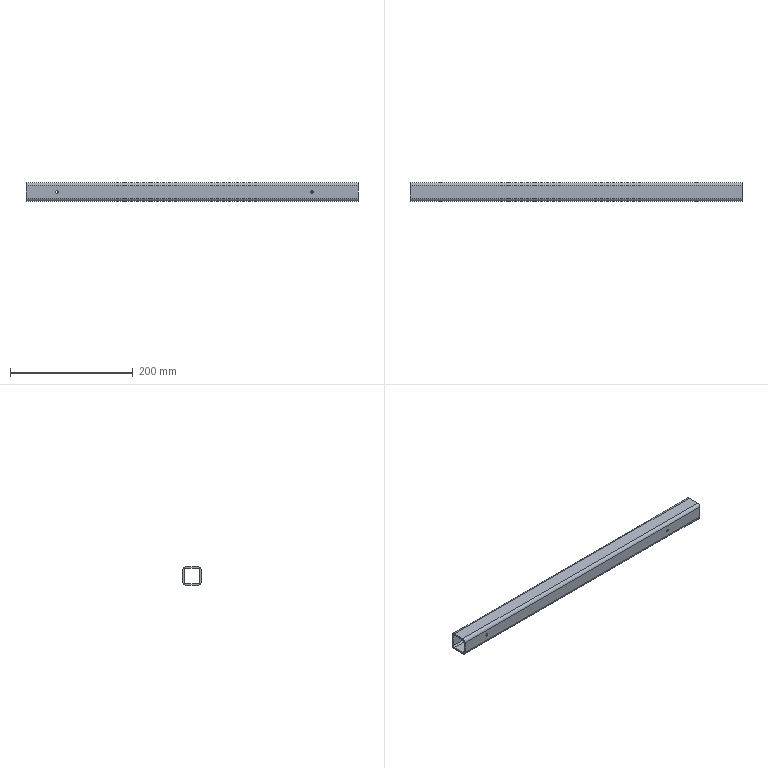Part | SolidWorks | features HoleWzd 2, 3DProfileFeature 1, WeldMemberFeat 1, WeldmentFeature 1 | 1 solid | 26 faces | box 540 x 30 x 30 mm | volume 144334 mm3 | cylinder 16 | plane 10 | commonest cylinder face diameters 4.2 x8 5.2 x4 10.4 x4
STEP:
#1=CARTESIAN_POINT('',(50.,15.,2.1));
#2=VERTEX_POINT('',#1);
#3=CARTESIAN_POINT('',(50.,15.,-2.1));
#4=VERTEX_POINT('',#3);
#5=CARTESIAN_POINT('',(50.,15.,0.));
#6=DIRECTION('',(0.,-1.,0.));
#7=DIRECTION('',(0.,0.,-1.));
#8=AXIS2_PLACEMENT_3D('',#5,#6,#7);
#9=CIRCLE('',#8,2.1);
#10=EDGE_CURVE('',#2,#4,#9,.T.);
#11=ORIENTED_EDGE('',*,*,#10,.F.);
#12=CARTESIAN_POINT('',(50.,12.4,2.1));
#13=VERTEX_POINT('',#12);
#14=CARTESIAN_POINT('',(50.,-15.,2.1));
#15=DIRECTION('',(0.,-1.,0.));
#16=VECTOR('',#15,1000.);
#17=LINE('',#14,#16);
#18=EDGE_CURVE('',#2,#13,#17,.T.);
#19=ORIENTED_EDGE('',*,*,#18,.T.);
#20=CARTESIAN_POINT('',(50.,12.4,-2.1));
#21=VERTEX_POINT('',#20);
#22=CARTESIAN_POINT('',(50.,12.4,0.));
#23=DIRECTION('',(0.,-1.,0.));
#24=DIRECTION('',(0.,0.,-1.));
#25=AXIS2_PLACEMENT_3D('',#22,#23,#24);
#26=CIRCLE('',#25,2.1);
#27=EDGE_CURVE('',#13,#21,#26,.T.);
#28=ORIENTED_EDGE('',*,*,#27,.T.);
#29=CARTESIAN_POINT('',(50.,-15.,-2.1));
#30=DIRECTION('',(0.,-1.,0.));
#31=VECTOR('',#30,1000.);
#32=LINE('',#29,#31);
#33=EDGE_CURVE('',#4,#21,#32,.T.);
#34=ORIENTED_EDGE('',*,*,#33,.F.);
#35=EDGE_LOOP('',(#11,#19,#28,#34));
#36=FACE_OUTER_BOUND('',#35,.T.);
#37=CARTESIAN_POINT('',(50.,-15.,0.));
#38=DIRECTION('',(0.,-1.,0.));
#39=DIRECTION('',(0.,0.,-1.));
#40=AXIS2_PLACEMENT_3D('',#37,#38,#39);
#41=CYLINDRICAL_SURFACE('',#40,2.1);
#42=ADVANCED_FACE('',(#36),#41,.F.);
#43=CARTESIAN_POINT('',(50.,-12.4,-2.1));
#44=VERTEX_POINT('',#43);
#45=CARTESIAN_POINT('',(50.,-12.4,2.1));
#46=VERTEX_POINT('',#45);
#47=CARTESIAN_POINT('',(50.,-12.4,0.));
#48=DIRECTION('',(0.,1.,0.));
#49=DIRECTION('',(0.,0.,1.));
#50=AXIS2_PLACEMENT_3D('',#47,#48,#49);
#51=CIRCLE('',#50,2.1);
#52=EDGE_CURVE('',#44,#46,#51,.T.);
#53=ORIENTED_EDGE('',*,*,#52,.T.);
#54=CARTESIAN_POINT('',(50.,-15.,2.1));
#55=VERTEX_POINT('',#54);
#56=CARTESIAN_POINT('',(50.,-15.,2.1));
#57=DIRECTION('',(0.,-1.,0.));
#58=VECTOR('',#57,1000.);
#59=LINE('',#56,#58);
#60=EDGE_CURVE('',#46,#55,#59,.T.);
#61=ORIENTED_EDGE('',*,*,#60,.T.);
#62=CARTESIAN_POINT('',(50.,-15.,-2.1));
#63=VERTEX_POINT('',#62);
#64=CARTESIAN_POINT('',(50.,-15.,0.));
#65=DIRECTION('',(0.,-1.,0.));
#66=DIRECTION('',(0.,0.,-1.));
#67=AXIS2_PLACEMENT_3D('',#64,#65,#66);
#68=CIRCLE('',#67,2.1);
#69=EDGE_CURVE('',#55,#63,#68,.T.);
#70=ORIENTED_EDGE('',*,*,#69,.T.);
#71=CARTESIAN_POINT('',(50.,-15.,-2.1));
#72=DIRECTION('',(0.,-1.,0.));
#73=VECTOR('',#72,1000.);
#74=LINE('',#71,#73);
#75=EDGE_CURVE('',#44,#63,#74,.T.);
#76=ORIENTED_EDGE('',*,*,#75,.F.);
#77=EDGE_LOOP('',(#53,#61,#70,#76));
#78=FACE_OUTER_BOUND('',#77,.T.);
#79=CARTESIAN_POINT('',(50.,-15.,0.));
#80=DIRECTION('',(0.,-1.,0.));
#81=DIRECTION('',(0.,0.,-1.));
#82=AXIS2_PLACEMENT_3D('',#79,#80,#81);
#83=CYLINDRICAL_SURFACE('',#82,2.1);
#84=ADVANCED_FACE('',(#78),#83,.F.);
#85=CARTESIAN_POINT('',(465.,15.,2.1));
#86=VERTEX_POINT('',#85);
#87=CARTESIAN_POINT('',(465.,15.,-2.1));
#88=VERTEX_POINT('',#87);
#89=CARTESIAN_POINT('',(465.,15.,0.));
#90=DIRECTION('',(0.,-1.,0.));
#91=DIRECTION('',(0.,0.,-1.));
#92=AXIS2_PLACEMENT_3D('',#89,#90,#91);
#93=CIRCLE('',#92,2.1);
#94=EDGE_CURVE('',#86,#88,#93,.T.);
#95=ORIENTED_EDGE('',*,*,#94,.F.);
#96=CARTESIAN_POINT('',(465.,12.4,2.1));
#97=VERTEX_POINT('',#96);
#98=CARTESIAN_POINT('',(465.,-15.,2.1));
#99=DIRECTION('',(0.,-1.,0.));
#100=VECTOR('',#99,1000.);
#101=LINE('',#98,#100);
#102=EDGE_CURVE('',#86,#97,#101,.T.);
#103=ORIENTED_EDGE('',*,*,#102,.T.);
#104=CARTESIAN_POINT('',(465.,12.4,-2.1));
#105=VERTEX_POINT('',#104);
#106=CARTESIAN_POINT('',(465.,12.4,0.));
#107=DIRECTION('',(0.,-1.,0.));
#108=DIRECTION('',(0.,0.,-1.));
#109=AXIS2_PLACEMENT_3D('',#106,#107,#108);
#110=CIRCLE('',#109,2.1);
#111=EDGE_CURVE('',#97,#105,#110,.T.);
#112=ORIENTED_EDGE('',*,*,#111,.T.);
#113=CARTESIAN_POINT('',(465.,-15.,-2.1));
#114=DIRECTION('',(0.,-1.,0.));
#115=VECTOR('',#114,1000.);
#116=LINE('',#113,#115);
#117=EDGE_CURVE('',#88,#105,#116,.T.);
#118=ORIENTED_EDGE('',*,*,#117,.F.);
#119=EDGE_LOOP('',(#95,#103,#112,#118));
#120=FACE_OUTER_BOUND('',#119,.T.);
#121=CARTESIAN_POINT('',(465.,-15.,0.));
#122=DIRECTION('',(0.,-1.,0.));
#123=DIRECTION('',(0.,0.,-1.));
#124=AXIS2_PLACEMENT_3D('',#121,#122,#123);
#125=CYLINDRICAL_SURFACE('',#124,2.1);
#126=ADVANCED_FACE('',(#120),#125,.F.);
#127=CARTESIAN_POINT('',(465.,-12.4,-2.1));
#128=VERTEX_POINT('',#127);
#129=CARTESIAN_POINT('',(465.,-12.4,2.1));
#130=VERTEX_POINT('',#129);
#131=CARTESIAN_POINT('',(465.,-12.4,0.));
#132=DIRECTION('',(0.,1.,0.));
#133=DIRECTION('',(0.,0.,1.));
#134=AXIS2_PLACEMENT_3D('',#131,#132,#133);
#135=CIRCLE('',#134,2.1);
#136=EDGE_CURVE('',#128,#130,#135,.T.);
#137=ORIENTED_EDGE('',*,*,#136,.T.);
#138=CARTESIAN_POINT('',(465.,-15.,2.1));
#139=VERTEX_POINT('',#138);
#140=CARTESIAN_POINT('',(465.,-15.,2.1));
#141=DIRECTION('',(0.,-1.,0.));
#142=VECTOR('',#141,1000.);
#143=LINE('',#140,#142);
#144=EDGE_CURVE('',#130,#139,#143,.T.);
#145=ORIENTED_EDGE('',*,*,#144,.T.);
#146=CARTESIAN_POINT('',(465.,-15.,-2.1));
#147=VERTEX_POINT('',#146);
#148=CARTESIAN_POINT('',(465.,-15.,0.));
#149=DIRECTION('',(0.,-1.,0.));
#150=DIRECTION('',(0.,0.,-1.));
#151=AXIS2_PLACEMENT_3D('',#148,#149,#150);
#152=CIRCLE('',#151,2.1);
#153=EDGE_CURVE('',#139,#147,#152,.T.);
#154=ORIENTED_EDGE('',*,*,#153,.T.);
#155=CARTESIAN_POINT('',(465.,-15.,-2.1));
#156=DIRECTION('',(0.,-1.,0.));
#157=VECTOR('',#156,1000.);
#158=LINE('',#155,#157);
#159=EDGE_CURVE('',#128,#147,#158,.T.);
#160=ORIENTED_EDGE('',*,*,#159,.F.);
#161=EDGE_LOOP('',(#137,#145,#154,#160));
#162=FACE_OUTER_BOUND('',#161,.T.);
#163=CARTESIAN_POINT('',(465.,-15.,0.));
#164=DIRECTION('',(0.,-1.,0.));
#165=DIRECTION('',(0.,0.,-1.));
#166=AXIS2_PLACEMENT_3D('',#163,#164,#165);
#167=CYLINDRICAL_SURFACE('',#166,2.1);
#168=ADVANCED_FACE('',(#162),#167,.F.);
#169=CARTESIAN_POINT('',(0.,9.8,-15.));
#170=VERTEX_POINT('',#169);
#171=CARTESIAN_POINT('',(0.,15.,-9.8));
#172=VERTEX_POINT('',#171);
#173=CARTESIAN_POINT('',(0.,9.8,-9.8));
#174=DIRECTION('',(1.,0.,0.));
#175=DIRECTION('',(0.,0.,-1.));
#176=AXIS2_PLACEMENT_3D('',#173,#174,#175);
#177=CIRCLE('',#176,5.2);
#178=EDGE_CURVE('',#170,#172,#177,.T.);
#179=ORIENTED_EDGE('',*,*,#178,.T.);
#180=CARTESIAN_POINT('',(540.,15.,-9.8));
#181=VERTEX_POINT('',#180);
#182=CARTESIAN_POINT('',(540.,15.,-9.8));
#183=DIRECTION('',(-1.,0.,0.));
#184=VECTOR('',#183,1000.);
#185=LINE('',#182,#184);
#186=EDGE_CURVE('',#181,#172,#185,.T.);
#187=ORIENTED_EDGE('',*,*,#186,.F.);
#188=CARTESIAN_POINT('',(540.,9.8,-15.));
#189=VERTEX_POINT('',#188);
#190=CARTESIAN_POINT('',(540.,9.8,-9.8));
#191=DIRECTION('',(1.,0.,0.));
#192=DIRECTION('',(0.,0.,-1.));
#193=AXIS2_PLACEMENT_3D('',#190,#191,#192);
#194=CIRCLE('',#193,5.2);
#195=EDGE_CURVE('',#189,#181,#194,.T.);
#196=ORIENTED_EDGE('',*,*,#195,.F.);
#197=CARTESIAN_POINT('',(540.,9.8,-15.));
#198=DIRECTION('',(-1.,0.,0.));
#199=VECTOR('',#198,1000.);
#200=LINE('',#197,#199);
#201=EDGE_CURVE('',#189,#170,#200,.T.);
#202=ORIENTED_EDGE('',*,*,#201,.T.);
#203=EDGE_LOOP('',(#179,#187,#196,#202));
#204=FACE_OUTER_BOUND('',#203,.T.);
#205=CARTESIAN_POINT('',(540.,9.8,-9.8));
#206=DIRECTION('',(-1.,0.,0.));
#207=DIRECTION('',(0.,0.,1.));
#208=AXIS2_PLACEMENT_3D('',#205,#206,#207);
#209=CYLINDRICAL_SURFACE('',#208,5.2);
#210=ADVANCED_FACE('',(#204),#209,.T.);
#211=CARTESIAN_POINT('',(50.,15.,0.));
#212=DIRECTION('',(0.,-1.,0.));
#213=DIRECTION('',(0.,0.,-1.));
#214=AXIS2_PLACEMENT_3D('',#211,#212,#213);
#215=CIRCLE('',#214,2.1);
#216=EDGE_CURVE('',#4,#2,#215,.T.);
#217=ORIENTED_EDGE('',*,*,#216,.T.);
#218=ORIENTED_EDGE('',*,*,#10,.T.);
#219=EDGE_LOOP('',(#217,#218));
#220=FACE_BOUND('',#219,.T.);
#221=CARTESIAN_POINT('',(465.,15.,0.));
#222=DIRECTION('',(0.,-1.,0.));
#223=DIRECTION('',(0.,0.,-1.));
#224=AXIS2_PLACEMENT_3D('',#221,#222,#223);
#225=CIRCLE('',#224,2.1);
#226=EDGE_CURVE('',#88,#86,#225,.T.);
#227=ORIENTED_EDGE('',*,*,#226,.T.);
#228=ORIENTED_EDGE('',*,*,#94,.T.);
#229=EDGE_LOOP('',(#227,#228));
#230=FACE_BOUND('',#229,.T.);
#231=CARTESIAN_POINT('',(0.,15.,9.8));
#232=VERTEX_POINT('',#231);
#233=CARTESIAN_POINT('',(0.,15.,-9.8));
#234=DIRECTION('',(0.,0.,1.));
#235=VECTOR('',#234,1000.);
#236=LINE('',#233,#235);
#237=EDGE_CURVE('',#172,#232,#236,.T.);
#238=ORIENTED_EDGE('',*,*,#237,.T.);
#239=CARTESIAN_POINT('',(540.,15.,9.8));
#240=VERTEX_POINT('',#239);
#241=CARTESIAN_POINT('',(540.,15.,9.8));
#242=DIRECTION('',(-1.,0.,0.));
#243=VECTOR('',#242,1000.);
#244=LINE('',#241,#243);
#245=EDGE_CURVE('',#240,#232,#244,.T.);
#246=ORIENTED_EDGE('',*,*,#245,.F.);
#247=CARTESIAN_POINT('',(540.,15.,-9.8));
#248=DIRECTION('',(0.,0.,1.));
#249=VECTOR('',#248,1000.);
#250=LINE('',#247,#249);
#251=EDGE_CURVE('',#181,#240,#250,.T.);
#252=ORIENTED_EDGE('',*,*,#251,.F.);
#253=ORIENTED_EDGE('',*,*,#186,.T.);
#254=EDGE_LOOP('',(#238,#246,#252,#253));
#255=FACE_OUTER_BOUND('',#254,.T.);
#256=CARTESIAN_POINT('',(540.,15.,-9.8));
#257=DIRECTION('',(0.,-1.,0.));
#258=DIRECTION('',(0.,0.,-1.));
#259=AXIS2_PLACEMENT_3D('',#256,#257,#258);
#260=PLANE('',#259);
#261=ADVANCED_FACE('',(#220,#230,#255),#260,.F.);
#262=CARTESIAN_POINT('',(0.,9.8,15.));
#263=VERTEX_POINT('',#262);
#264=CARTESIAN_POINT('',(0.,9.8,9.8));
#265=DIRECTION('',(1.,0.,0.));
#266=DIRECTION('',(0.,0.,-1.));
#267=AXIS2_PLACEMENT_3D('',#264,#265,#266);
#268=CIRCLE('',#267,5.2);
#269=EDGE_CURVE('',#232,#263,#268,.T.);
#270=ORIENTED_EDGE('',*,*,#269,.T.);
#271=CARTESIAN_POINT('',(540.,9.8,15.));
#272=VERTEX_POINT('',#271);
#273=CARTESIAN_POINT('',(540.,9.8,15.));
#274=DIRECTION('',(-1.,0.,0.));
#275=VECTOR('',#274,1000.);
#276=LINE('',#273,#275);
#277=EDGE_CURVE('',#272,#263,#276,.T.);
#278=ORIENTED_EDGE('',*,*,#277,.F.);
#279=CARTESIAN_POINT('',(540.,9.8,9.8));
#280=DIRECTION('',(1.,0.,0.));
#281=DIRECTION('',(0.,0.,-1.));
#282=AXIS2_PLACEMENT_3D('',#279,#280,#281);
#283=CIRCLE('',#282,5.2);
#284=EDGE_CURVE('',#240,#272,#283,.T.);
#285=ORIENTED_EDGE('',*,*,#284,.F.);
#286=ORIENTED_EDGE('',*,*,#245,.T.);
#287=EDGE_LOOP('',(#270,#278,#285,#286));
#288=FACE_OUTER_BOUND('',#287,.T.);
#289=CARTESIAN_POINT('',(540.,9.8,9.8));
#290=DIRECTION('',(-1.,0.,0.));
#291=DIRECTION('',(0.,0.,1.));
#292=AXIS2_PLACEMENT_3D('',#289,#290,#291);
#293=CYLINDRICAL_SURFACE('',#292,5.2);
#294=ADVANCED_FACE('',(#288),#293,.T.);
#295=CARTESIAN_POINT('',(0.,-9.8,15.));
#296=VERTEX_POINT('',#295);
#297=CARTESIAN_POINT('',(0.,-9.8,15.));
#298=DIRECTION('',(0.,-1.,0.));
#299=VECTOR('',#298,1000.);
#300=LINE('',#297,#299);
#301=EDGE_CURVE('',#263,#296,#300,.T.);
#302=ORIENTED_EDGE('',*,*,#301,.T.);
#303=CARTESIAN_POINT('',(540.,-9.8,15.));
#304=VERTEX_POINT('',#303);
#305=CARTESIAN_POINT('',(540.,-9.8,15.));
#306=DIRECTION('',(-1.,0.,0.));
#307=VECTOR('',#306,1000.);
#308=LINE('',#305,#307);
#309=EDGE_CURVE('',#304,#296,#308,.T.);
#310=ORIENTED_EDGE('',*,*,#309,.F.);
#311=CARTESIAN_POINT('',(540.,-9.8,15.));
#312=DIRECTION('',(0.,-1.,0.));
#313=VECTOR('',#312,1000.);
#314=LINE('',#311,#313);
#315=EDGE_CURVE('',#272,#304,#314,.T.);
#316=ORIENTED_EDGE('',*,*,#315,.F.);
#317=ORIENTED_EDGE('',*,*,#277,.T.);
#318=EDGE_LOOP('',(#302,#310,#316,#317));
#319=FACE_OUTER_BOUND('',#318,.T.);
#320=CARTESIAN_POINT('',(540.,-9.8,15.));
#321=DIRECTION('',(0.,0.,-1.));
#322=DIRECTION('',(-1.,0.,0.));
#323=AXIS2_PLACEMENT_3D('',#320,#321,#322);
#324=PLANE('',#323);
#325=ADVANCED_FACE('',(#319),#324,.F.);
#326=CARTESIAN_POINT('',(0.,-15.,9.8));
#327=VERTEX_POINT('',#326);
#328=CARTESIAN_POINT('',(0.,-9.8,9.8));
#329=DIRECTION('',(1.,0.,0.));
#330=DIRECTION('',(0.,0.,-1.));
#331=AXIS2_PLACEMENT_3D('',#328,#329,#330);
#332=CIRCLE('',#331,5.2);
#333=EDGE_CURVE('',#296,#327,#332,.T.);
#334=ORIENTED_EDGE('',*,*,#333,.T.);
#335=CARTESIAN_POINT('',(540.,-15.,9.8));
#336=VERTEX_POINT('',#335);
#337=CARTESIAN_POINT('',(540.,-15.,9.8));
#338=DIRECTION('',(-1.,0.,0.));
#339=VECTOR('',#338,1000.);
#340=LINE('',#337,#339);
#341=EDGE_CURVE('',#336,#327,#340,.T.);
#342=ORIENTED_EDGE('',*,*,#341,.F.);
#343=CARTESIAN_POINT('',(540.,-9.8,9.8));
#344=DIRECTION('',(1.,0.,0.));
#345=DIRECTION('',(0.,0.,-1.));
#346=AXIS2_PLACEMENT_3D('',#343,#344,#345);
#347=CIRCLE('',#346,5.2);
#348=EDGE_CURVE('',#304,#336,#347,.T.);
#349=ORIENTED_EDGE('',*,*,#348,.F.);
#350=ORIENTED_EDGE('',*,*,#309,.T.);
#351=EDGE_LOOP('',(#334,#342,#349,#350));
#352=FACE_OUTER_BOUND('',#351,.T.);
#353=CARTESIAN_POINT('',(540.,-9.8,9.8));
#354=DIRECTION('',(-1.,0.,0.));
#355=DIRECTION('',(0.,0.,1.));
#356=AXIS2_PLACEMENT_3D('',#353,#354,#355);
#357=CYLINDRICAL_SURFACE('',#356,5.2);
#358=ADVANCED_FACE('',(#352),#357,.T.);
#359=CARTESIAN_POINT('',(50.,-15.,0.));
#360=DIRECTION('',(0.,-1.,0.));
#361=DIRECTION('',(0.,0.,-1.));
#362=AXIS2_PLACEMENT_3D('',#359,#360,#361);
#363=CIRCLE('',#362,2.1);
#364=EDGE_CURVE('',#63,#55,#363,.T.);
#365=ORIENTED_EDGE('',*,*,#364,.F.);
#366=ORIENTED_EDGE('',*,*,#69,.F.);
#367=EDGE_LOOP('',(#365,#366));
#368=FACE_BOUND('',#367,.T.);
#369=CARTESIAN_POINT('',(465.,-15.,0.));
#370=DIRECTION('',(0.,-1.,0.));
#371=DIRECTION('',(0.,0.,-1.));
#372=AXIS2_PLACEMENT_3D('',#369,#370,#371);
#373=CIRCLE('',#372,2.1);
#374=EDGE_CURVE('',#147,#139,#373,.T.);
#375=ORIENTED_EDGE('',*,*,#374,.F.);
#376=ORIENTED_EDGE('',*,*,#153,.F.);
#377=EDGE_LOOP('',(#375,#376));
#378=FACE_BOUND('',#377,.T.);
#379=CARTESIAN_POINT('',(0.,-15.,-9.8));
#380=VERTEX_POINT('',#379);
#381=CARTESIAN_POINT('',(0.,-15.,9.8));
#382=DIRECTION('',(0.,0.,-1.));
#383=VECTOR('',#382,1000.);
#384=LINE('',#381,#383);
#385=EDGE_CURVE('',#327,#380,#384,.T.);
#386=ORIENTED_EDGE('',*,*,#385,.T.);
#387=CARTESIAN_POINT('',(540.,-15.,-9.8));
#388=VERTEX_POINT('',#387);
#389=CARTESIAN_POINT('',(540.,-15.,-9.8));
#390=DIRECTION('',(-1.,0.,0.));
#391=VECTOR('',#390,1000.);
#392=LINE('',#389,#391);
#393=EDGE_CURVE('',#388,#380,#392,.T.);
#394=ORIENTED_EDGE('',*,*,#393,.F.);
#395=CARTESIAN_POINT('',(540.,-15.,9.8));
#396=DIRECTION('',(0.,0.,-1.));
#397=VECTOR('',#396,1000.);
#398=LINE('',#395,#397);
#399=EDGE_CURVE('',#336,#388,#398,.T.);
#400=ORIENTED_EDGE('',*,*,#399,.F.);
#401=ORIENTED_EDGE('',*,*,#341,.T.);
#402=EDGE_LOOP('',(#386,#394,#400,#401));
#403=FACE_OUTER_BOUND('',#402,.T.);
#404=CARTESIAN_POINT('',(540.,-15.,9.8));
#405=DIRECTION('',(0.,1.,0.));
#406=DIRECTION('',(0.,0.,1.));
#407=AXIS2_PLACEMENT_3D('',#404,#405,#406);
#408=PLANE('',#407);
#409=ADVANCED_FACE('',(#368,#378,#403),#408,.F.);
#410=CARTESIAN_POINT('',(0.,-9.8,-15.));
#411=VERTEX_POINT('',#410);
#412=CARTESIAN_POINT('',(0.,-9.8,-9.8));
#413=DIRECTION('',(1.,0.,0.));
#414=DIRECTION('',(0.,0.,-1.));
#415=AXIS2_PLACEMENT_3D('',#412,#413,#414);
#416=CIRCLE('',#415,5.2);
#417=EDGE_CURVE('',#380,#411,#416,.T.);
#418=ORIENTED_EDGE('',*,*,#417,.T.);
#419=CARTESIAN_POINT('',(540.,-9.8,-15.));
#420=VERTEX_POINT('',#419);
#421=CARTESIAN_POINT('',(540.,-9.8,-15.));
#422=DIRECTION('',(-1.,0.,0.));
#423=VECTOR('',#422,1000.);
#424=LINE('',#421,#423);
#425=EDGE_CURVE('',#420,#411,#424,.T.);
#426=ORIENTED_EDGE('',*,*,#425,.F.);
#427=CARTESIAN_POINT('',(540.,-9.8,-9.8));
#428=DIRECTION('',(1.,0.,0.));
#429=DIRECTION('',(0.,0.,-1.));
#430=AXIS2_PLACEMENT_3D('',#427,#428,#429);
#431=CIRCLE('',#430,5.2);
#432=EDGE_CURVE('',#388,#420,#431,.T.);
#433=ORIENTED_EDGE('',*,*,#432,.F.);
#434=ORIENTED_EDGE('',*,*,#393,.T.);
#435=EDGE_LOOP('',(#418,#426,#433,#434));
#436=FACE_OUTER_BOUND('',#435,.T.);
#437=CARTESIAN_POINT('',(540.,-9.8,-9.8));
#438=DIRECTION('',(-1.,0.,0.));
#439=DIRECTION('',(0.,0.,1.));
#440=AXIS2_PLACEMENT_3D('',#437,#438,#439);
#441=CYLINDRICAL_SURFACE('',#440,5.2);
#442=ADVANCED_FACE('',(#436),#441,.T.);
#443=CARTESIAN_POINT('',(0.,12.4,9.8));
#444=VERTEX_POINT('',#443);
#445=CARTESIAN_POINT('',(0.,9.8,12.4));
#446=VERTEX_POINT('',#445);
#447=CARTESIAN_POINT('',(0.,9.8,9.8));
#448=DIRECTION('',(1.,0.,0.));
#449=DIRECTION('',(0.,0.,-1.));
#450=AXIS2_PLACEMENT_3D('',#447,#448,#449);
#451=CIRCLE('',#450,2.6);
#452=EDGE_CURVE('',#444,#446,#451,.T.);
#453=ORIENTED_EDGE('',*,*,#452,.F.);
#454=CARTESIAN_POINT('',(540.,12.4,9.8));
#455=VERTEX_POINT('',#454);
#456=CARTESIAN_POINT('',(540.,12.4,9.8));
#457=DIRECTION('',(-1.,0.,0.));
#458=VECTOR('',#457,1000.);
#459=LINE('',#456,#458);
#460=EDGE_CURVE('',#455,#444,#459,.T.);
#461=ORIENTED_EDGE('',*,*,#460,.F.);
#462=CARTESIAN_POINT('',(540.,9.8,12.4));
#463=VERTEX_POINT('',#462);
#464=CARTESIAN_POINT('',(540.,9.8,9.8));
#465=DIRECTION('',(1.,0.,0.));
#466=DIRECTION('',(0.,0.,-1.));
#467=AXIS2_PLACEMENT_3D('',#464,#465,#466);
#468=CIRCLE('',#467,2.6);
#469=EDGE_CURVE('',#455,#463,#468,.T.);
#470=ORIENTED_EDGE('',*,*,#469,.T.);
#471=CARTESIAN_POINT('',(540.,9.8,12.4));
#472=DIRECTION('',(-1.,0.,0.));
#473=VECTOR('',#472,1000.);
#474=LINE('',#471,#473);
#475=EDGE_CURVE('',#463,#446,#474,.T.);
#476=ORIENTED_EDGE('',*,*,#475,.T.);
#477=EDGE_LOOP('',(#453,#461,#470,#476));
#478=FACE_OUTER_BOUND('',#477,.T.);
#479=CARTESIAN_POINT('',(540.,9.8,9.8));
#480=DIRECTION('',(-1.,0.,0.));
#481=DIRECTION('',(0.,0.,1.));
#482=AXIS2_PLACEMENT_3D('',#479,#480,#481);
#483=CYLINDRICAL_SURFACE('',#482,2.6);
#484=ADVANCED_FACE('',(#478),#483,.F.);
#485=CARTESIAN_POINT('',(50.,12.4,0.));
#486=DIRECTION('',(0.,-1.,0.));
#487=DIRECTION('',(0.,0.,-1.));
#488=AXIS2_PLACEMENT_3D('',#485,#486,#487);
#489=CIRCLE('',#488,2.1);
#490=EDGE_CURVE('',#21,#13,#489,.T.);
#491=ORIENTED_EDGE('',*,*,#490,.F.);
#492=ORIENTED_EDGE('',*,*,#27,.F.);
#493=EDGE_LOOP('',(#491,#492));
#494=FACE_BOUND('',#493,.T.);
#495=CARTESIAN_POINT('',(465.,12.4,0.));
#496=DIRECTION('',(0.,-1.,0.));
#497=DIRECTION('',(0.,0.,-1.));
#498=AXIS2_PLACEMENT_3D('',#495,#496,#497);
#499=CIRCLE('',#498,2.1);
#500=EDGE_CURVE('',#105,#97,#499,.T.);
#501=ORIENTED_EDGE('',*,*,#500,.F.);
#502=ORIENTED_EDGE('',*,*,#111,.F.);
#503=EDGE_LOOP('',(#501,#502));
#504=FACE_BOUND('',#503,.T.);
#505=CARTESIAN_POINT('',(0.,12.4,-9.8));
#506=VERTEX_POINT('',#505);
#507=CARTESIAN_POINT('',(0.,12.4,-9.8));
#508=DIRECTION('',(0.,0.,1.));
#509=VECTOR('',#508,1000.);
#510=LINE('',#507,#509);
#511=EDGE_CURVE('',#506,#444,#510,.T.);
#512=ORIENTED_EDGE('',*,*,#511,.F.);
#513=CARTESIAN_POINT('',(540.,12.4,-9.8));
#514=VERTEX_POINT('',#513);
#515=CARTESIAN_POINT('',(540.,12.4,-9.8));
#516=DIRECTION('',(-1.,0.,0.));
#517=VECTOR('',#516,1000.);
#518=LINE('',#515,#517);
#519=EDGE_CURVE('',#514,#506,#518,.T.);
#520=ORIENTED_EDGE('',*,*,#519,.F.);
#521=CARTESIAN_POINT('',(540.,12.4,-9.8));
#522=DIRECTION('',(0.,0.,1.));
#523=VECTOR('',#522,1000.);
#524=LINE('',#521,#523);
#525=EDGE_CURVE('',#514,#455,#524,.T.);
#526=ORIENTED_EDGE('',*,*,#525,.T.);
#527=ORIENTED_EDGE('',*,*,#460,.T.);
#528=EDGE_LOOP('',(#512,#520,#526,#527));
#529=FACE_OUTER_BOUND('',#528,.T.);
#530=CARTESIAN_POINT('',(540.,12.4,-9.8));
#531=DIRECTION('',(0.,-1.,0.));
#532=DIRECTION('',(0.,0.,-1.));
#533=AXIS2_PLACEMENT_3D('',#530,#531,#532);
#534=PLANE('',#533);
#535=ADVANCED_FACE('',(#494,#504,#529),#534,.T.);
#536=CARTESIAN_POINT('',(0.,9.8,-12.4));
#537=VERTEX_POINT('',#536);
#538=CARTESIAN_POINT('',(0.,9.8,-9.8));
#539=DIRECTION('',(1.,0.,0.));
#540=DIRECTION('',(0.,0.,-1.));
#541=AXIS2_PLACEMENT_3D('',#538,#539,#540);
#542=CIRCLE('',#541,2.6);
#543=EDGE_CURVE('',#537,#506,#542,.T.);
#544=ORIENTED_EDGE('',*,*,#543,.F.);
#545=CARTESIAN_POINT('',(540.,9.8,-12.4));
#546=VERTEX_POINT('',#545);
#547=CARTESIAN_POINT('',(540.,9.8,-12.4));
#548=DIRECTION('',(-1.,0.,0.));
#549=VECTOR('',#548,1000.);
#550=LINE('',#547,#549);
#551=EDGE_CURVE('',#546,#537,#550,.T.);
#552=ORIENTED_EDGE('',*,*,#551,.F.);
#553=CARTESIAN_POINT('',(540.,9.8,-9.8));
#554=DIRECTION('',(1.,0.,0.));
#555=DIRECTION('',(0.,0.,-1.));
#556=AXIS2_PLACEMENT_3D('',#553,#554,#555);
#557=CIRCLE('',#556,2.6);
#558=EDGE_CURVE('',#546,#514,#557,.T.);
#559=ORIENTED_EDGE('',*,*,#558,.T.);
#560=ORIENTED_EDGE('',*,*,#519,.T.);
#561=EDGE_LOOP('',(#544,#552,#559,#560));
#562=FACE_OUTER_BOUND('',#561,.T.);
#563=CARTESIAN_POINT('',(540.,9.8,-9.8));
#564=DIRECTION('',(-1.,0.,0.));
#565=DIRECTION('',(0.,0.,1.));
#566=AXIS2_PLACEMENT_3D('',#563,#564,#565);
#567=CYLINDRICAL_SURFACE('',#566,2.6);
#568=ADVANCED_FACE('',(#562),#567,.F.);
#569=CARTESIAN_POINT('',(0.,-9.8,-12.4));
#570=VERTEX_POINT('',#569);
#571=CARTESIAN_POINT('',(0.,9.8,-12.4));
#572=DIRECTION('',(0.,1.,0.));
#573=VECTOR('',#572,1000.);
#574=LINE('',#571,#573);
#575=EDGE_CURVE('',#570,#537,#574,.T.);
#576=ORIENTED_EDGE('',*,*,#575,.F.);
#577=CARTESIAN_POINT('',(540.,-9.8,-12.4));
#578=VERTEX_POINT('',#577);
#579=CARTESIAN_POINT('',(540.,-9.8,-12.4));
#580=DIRECTION('',(-1.,0.,0.));
#581=VECTOR('',#580,1000.);
#582=LINE('',#579,#581);
#583=EDGE_CURVE('',#578,#570,#582,.T.);
#584=ORIENTED_EDGE('',*,*,#583,.F.);
#585=CARTESIAN_POINT('',(540.,9.8,-12.4));
#586=DIRECTION('',(0.,1.,0.));
#587=VECTOR('',#586,1000.);
#588=LINE('',#585,#587);
#589=EDGE_CURVE('',#578,#546,#588,.T.);
#590=ORIENTED_EDGE('',*,*,#589,.T.);
#591=ORIENTED_EDGE('',*,*,#551,.T.);
#592=EDGE_LOOP('',(#576,#584,#590,#591));
#593=FACE_OUTER_BOUND('',#592,.T.);
#594=CARTESIAN_POINT('',(540.,9.8,-12.4));
#595=DIRECTION('',(0.,0.,1.));
#596=DIRECTION('',(1.,0.,0.));
#597=AXIS2_PLACEMENT_3D('',#594,#595,#596);
#598=PLANE('',#597);
#599=ADVANCED_FACE('',(#593),#598,.T.);
#600=CARTESIAN_POINT('',(0.,-12.4,-9.8));
#601=VERTEX_POINT('',#600);
#602=CARTESIAN_POINT('',(0.,-9.8,-9.8));
#603=DIRECTION('',(1.,0.,0.));
#604=DIRECTION('',(0.,0.,-1.));
#605=AXIS2_PLACEMENT_3D('',#602,#603,#604);
#606=CIRCLE('',#605,2.6);
#607=EDGE_CURVE('',#601,#570,#606,.T.);
#608=ORIENTED_EDGE('',*,*,#607,.F.);
#609=CARTESIAN_POINT('',(540.,-12.4,-9.8));
#610=VERTEX_POINT('',#609);
#611=CARTESIAN_POINT('',(540.,-12.4,-9.8));
#612=DIRECTION('',(-1.,0.,0.));
#613=VECTOR('',#612,1000.);
#614=LINE('',#611,#613);
#615=EDGE_CURVE('',#610,#601,#614,.T.);
#616=ORIENTED_EDGE('',*,*,#615,.F.);
#617=CARTESIAN_POINT('',(540.,-9.8,-9.8));
#618=DIRECTION('',(1.,0.,0.));
#619=DIRECTION('',(0.,0.,-1.));
#620=AXIS2_PLACEMENT_3D('',#617,#618,#619);
#621=CIRCLE('',#620,2.6);
#622=EDGE_CURVE('',#610,#578,#621,.T.);
#623=ORIENTED_EDGE('',*,*,#622,.T.);
#624=ORIENTED_EDGE('',*,*,#583,.T.);
#625=EDGE_LOOP('',(#608,#616,#623,#624));
#626=FACE_OUTER_BOUND('',#625,.T.);
#627=CARTESIAN_POINT('',(540.,-9.8,-9.8));
#628=DIRECTION('',(-1.,0.,0.));
#629=DIRECTION('',(0.,0.,1.));
#630=AXIS2_PLACEMENT_3D('',#627,#628,#629);
#631=CYLINDRICAL_SURFACE('',#630,2.6);
#632=ADVANCED_FACE('',(#626),#631,.F.);
#633=ORIENTED_EDGE('',*,*,#52,.F.);
#634=CARTESIAN_POINT('',(50.,-12.4,0.));
#635=DIRECTION('',(0.,1.,0.));
#636=DIRECTION('',(0.,0.,1.));
#637=AXIS2_PLACEMENT_3D('',#634,#635,#636);
#638=CIRCLE('',#637,2.1);
#639=EDGE_CURVE('',#46,#44,#638,.T.);
#640=ORIENTED_EDGE('',*,*,#639,.F.);
#641=EDGE_LOOP('',(#633,#640));
#642=FACE_BOUND('',#641,.T.);
#643=ORIENTED_EDGE('',*,*,#136,.F.);
#644=CARTESIAN_POINT('',(465.,-12.4,0.));
#645=DIRECTION('',(0.,1.,0.));
#646=DIRECTION('',(0.,0.,1.));
#647=AXIS2_PLACEMENT_3D('',#644,#645,#646);
#648=CIRCLE('',#647,2.1);
#649=EDGE_CURVE('',#130,#128,#648,.T.);
#650=ORIENTED_EDGE('',*,*,#649,.F.);
#651=EDGE_LOOP('',(#643,#650));
#652=FACE_BOUND('',#651,.T.);
#653=CARTESIAN_POINT('',(0.,-12.4,9.8));
#654=VERTEX_POINT('',#653);
#655=CARTESIAN_POINT('',(0.,-12.4,9.8));
#656=DIRECTION('',(0.,0.,-1.));
#657=VECTOR('',#656,1000.);
#658=LINE('',#655,#657);
#659=EDGE_CURVE('',#654,#601,#658,.T.);
#660=ORIENTED_EDGE('',*,*,#659,.F.);
#661=CARTESIAN_POINT('',(540.,-12.4,9.8));
#662=VERTEX_POINT('',#661);
#663=CARTESIAN_POINT('',(540.,-12.4,9.8));
#664=DIRECTION('',(-1.,0.,0.));
#665=VECTOR('',#664,1000.);
#666=LINE('',#663,#665);
#667=EDGE_CURVE('',#662,#654,#666,.T.);
#668=ORIENTED_EDGE('',*,*,#667,.F.);
#669=CARTESIAN_POINT('',(540.,-12.4,9.8));
#670=DIRECTION('',(0.,0.,-1.));
#671=VECTOR('',#670,1000.);
#672=LINE('',#669,#671);
#673=EDGE_CURVE('',#662,#610,#672,.T.);
#674=ORIENTED_EDGE('',*,*,#673,.T.);
#675=ORIENTED_EDGE('',*,*,#615,.T.);
#676=EDGE_LOOP('',(#660,#668,#674,#675));
#677=FACE_OUTER_BOUND('',#676,.T.);
#678=CARTESIAN_POINT('',(540.,-12.4,9.8));
#679=DIRECTION('',(0.,1.,0.));
#680=DIRECTION('',(0.,0.,1.));
#681=AXIS2_PLACEMENT_3D('',#678,#679,#680);
#682=PLANE('',#681);
#683=ADVANCED_FACE('',(#642,#652,#677),#682,.T.);
#684=CARTESIAN_POINT('',(0.,-9.8,12.4));
#685=VERTEX_POINT('',#684);
#686=CARTESIAN_POINT('',(0.,-9.8,9.8));
#687=DIRECTION('',(1.,0.,0.));
#688=DIRECTION('',(0.,0.,-1.));
#689=AXIS2_PLACEMENT_3D('',#686,#687,#688);
#690=CIRCLE('',#689,2.6);
#691=EDGE_CURVE('',#685,#654,#690,.T.);
#692=ORIENTED_EDGE('',*,*,#691,.F.);
#693=CARTESIAN_POINT('',(540.,-9.8,12.4));
#694=VERTEX_POINT('',#693);
#695=CARTESIAN_POINT('',(540.,-9.8,12.4));
#696=DIRECTION('',(-1.,0.,0.));
#697=VECTOR('',#696,1000.);
#698=LINE('',#695,#697);
#699=EDGE_CURVE('',#694,#685,#698,.T.);
#700=ORIENTED_EDGE('',*,*,#699,.F.);
#701=CARTESIAN_POINT('',(540.,-9.8,9.8));
#702=DIRECTION('',(1.,0.,0.));
#703=DIRECTION('',(0.,0.,-1.));
#704=AXIS2_PLACEMENT_3D('',#701,#702,#703);
#705=CIRCLE('',#704,2.6);
#706=EDGE_CURVE('',#694,#662,#705,.T.);
#707=ORIENTED_EDGE('',*,*,#706,.T.);
#708=ORIENTED_EDGE('',*,*,#667,.T.);
#709=EDGE_LOOP('',(#692,#700,#707,#708));
#710=FACE_OUTER_BOUND('',#709,.T.);
#711=CARTESIAN_POINT('',(540.,-9.8,9.8));
#712=DIRECTION('',(-1.,0.,0.));
#713=DIRECTION('',(0.,0.,1.));
#714=AXIS2_PLACEMENT_3D('',#711,#712,#713);
#715=CYLINDRICAL_SURFACE('',#714,2.6);
#716=ADVANCED_FACE('',(#710),#715,.F.);
#717=CARTESIAN_POINT('',(0.,-9.8,12.4));
#718=DIRECTION('',(0.,-1.,0.));
#719=VECTOR('',#718,1000.);
#720=LINE('',#717,#719);
#721=EDGE_CURVE('',#446,#685,#720,.T.);
#722=ORIENTED_EDGE('',*,*,#721,.F.);
#723=ORIENTED_EDGE('',*,*,#475,.F.);
#724=CARTESIAN_POINT('',(540.,-9.8,12.4));
#725=DIRECTION('',(0.,-1.,0.));
#726=VECTOR('',#725,1000.);
#727=LINE('',#724,#726);
#728=EDGE_CURVE('',#463,#694,#727,.T.);
#729=ORIENTED_EDGE('',*,*,#728,.T.);
#730=ORIENTED_EDGE('',*,*,#699,.T.);
#731=EDGE_LOOP('',(#722,#723,#729,#730));
#732=FACE_OUTER_BOUND('',#731,.T.);
#733=CARTESIAN_POINT('',(540.,-9.8,12.4));
#734=DIRECTION('',(0.,0.,-1.));
#735=DIRECTION('',(-1.,0.,0.));
#736=AXIS2_PLACEMENT_3D('',#733,#734,#735);
#737=PLANE('',#736);
#738=ADVANCED_FACE('',(#732),#737,.T.);
#739=CARTESIAN_POINT('',(0.,9.8,-15.));
#740=DIRECTION('',(0.,1.,0.));
#741=VECTOR('',#740,1000.);
#742=LINE('',#739,#741);
#743=EDGE_CURVE('',#411,#170,#742,.T.);
#744=ORIENTED_EDGE('',*,*,#743,.T.);
#745=ORIENTED_EDGE('',*,*,#201,.F.);
#746=CARTESIAN_POINT('',(540.,9.8,-15.));
#747=DIRECTION('',(0.,1.,0.));
#748=VECTOR('',#747,1000.);
#749=LINE('',#746,#748);
#750=EDGE_CURVE('',#420,#189,#749,.T.);
#751=ORIENTED_EDGE('',*,*,#750,.F.);
#752=ORIENTED_EDGE('',*,*,#425,.T.);
#753=EDGE_LOOP('',(#744,#745,#751,#752));
#754=FACE_OUTER_BOUND('',#753,.T.);
#755=CARTESIAN_POINT('',(540.,9.8,-15.));
#756=DIRECTION('',(0.,0.,1.));
#757=DIRECTION('',(1.,0.,0.));
#758=AXIS2_PLACEMENT_3D('',#755,#756,#757);
#759=PLANE('',#758);
#760=ADVANCED_FACE('',(#754),#759,.F.);
#761=ORIENTED_EDGE('',*,*,#469,.F.);
#762=ORIENTED_EDGE('',*,*,#525,.F.);
#763=ORIENTED_EDGE('',*,*,#558,.F.);
#764=ORIENTED_EDGE('',*,*,#589,.F.);
#765=ORIENTED_EDGE('',*,*,#622,.F.);
#766=ORIENTED_EDGE('',*,*,#673,.F.);
#767=ORIENTED_EDGE('',*,*,#706,.F.);
#768=ORIENTED_EDGE('',*,*,#728,.F.);
#769=EDGE_LOOP('',(#761,#762,#763,#764,#765,#766,#767,#768));
#770=FACE_BOUND('',#769,.T.);
#771=ORIENTED_EDGE('',*,*,#195,.T.);
#772=ORIENTED_EDGE('',*,*,#251,.T.);
#773=ORIENTED_EDGE('',*,*,#284,.T.);
#774=ORIENTED_EDGE('',*,*,#315,.T.);
#775=ORIENTED_EDGE('',*,*,#348,.T.);
#776=ORIENTED_EDGE('',*,*,#399,.T.);
#777=ORIENTED_EDGE('',*,*,#432,.T.);
#778=ORIENTED_EDGE('',*,*,#750,.T.);
#779=EDGE_LOOP('',(#771,#772,#773,#774,#775,#776,#777,#778));
#780=FACE_OUTER_BOUND('',#779,.T.);
#781=CARTESIAN_POINT('',(540.,9.8,-9.8));
#782=DIRECTION('',(1.,0.,0.));
#783=DIRECTION('',(0.,0.,-1.));
#784=AXIS2_PLACEMENT_3D('',#781,#782,#783);
#785=PLANE('',#784);
#786=ADVANCED_FACE('',(#770,#780),#785,.T.);
#787=ORIENTED_EDGE('',*,*,#452,.T.);
#788=ORIENTED_EDGE('',*,*,#721,.T.);
#789=ORIENTED_EDGE('',*,*,#691,.T.);
#790=ORIENTED_EDGE('',*,*,#659,.T.);
#791=ORIENTED_EDGE('',*,*,#607,.T.);
#792=ORIENTED_EDGE('',*,*,#575,.T.);
#793=ORIENTED_EDGE('',*,*,#543,.T.);
#794=ORIENTED_EDGE('',*,*,#511,.T.);
#795=EDGE_LOOP('',(#787,#788,#789,#790,#791,#792,#793,#794));
#796=FACE_BOUND('',#795,.T.);
#797=ORIENTED_EDGE('',*,*,#178,.F.);
#798=ORIENTED_EDGE('',*,*,#743,.F.);
#799=ORIENTED_EDGE('',*,*,#417,.F.);
#800=ORIENTED_EDGE('',*,*,#385,.F.);
#801=ORIENTED_EDGE('',*,*,#333,.F.);
#802=ORIENTED_EDGE('',*,*,#301,.F.);
#803=ORIENTED_EDGE('',*,*,#269,.F.);
#804=ORIENTED_EDGE('',*,*,#237,.F.);
#805=EDGE_LOOP('',(#797,#798,#799,#800,#801,#802,#803,#804));
#806=FACE_OUTER_BOUND('',#805,.T.);
#807=CARTESIAN_POINT('',(0.,9.8,-9.8));
#808=DIRECTION('',(1.,0.,0.));
#809=DIRECTION('',(0.,0.,-1.));
#810=AXIS2_PLACEMENT_3D('',#807,#808,#809);
#811=PLANE('',#810);
#812=ADVANCED_FACE('',(#796,#806),#811,.F.);
#813=ORIENTED_EDGE('',*,*,#144,.F.);
#814=ORIENTED_EDGE('',*,*,#649,.T.);
#815=ORIENTED_EDGE('',*,*,#159,.T.);
#816=ORIENTED_EDGE('',*,*,#374,.T.);
#817=EDGE_LOOP('',(#813,#814,#815,#816));
#818=FACE_OUTER_BOUND('',#817,.T.);
#819=CARTESIAN_POINT('',(465.,-15.,0.));
#820=DIRECTION('',(0.,-1.,0.));
#821=DIRECTION('',(0.,0.,-1.));
#822=AXIS2_PLACEMENT_3D('',#819,#820,#821);
#823=CYLINDRICAL_SURFACE('',#822,2.1);
#824=ADVANCED_FACE('',(#818),#823,.F.);
#825=ORIENTED_EDGE('',*,*,#102,.F.);
#826=ORIENTED_EDGE('',*,*,#226,.F.);
#827=ORIENTED_EDGE('',*,*,#117,.T.);
#828=ORIENTED_EDGE('',*,*,#500,.T.);
#829=EDGE_LOOP('',(#825,#826,#827,#828));
#830=FACE_OUTER_BOUND('',#829,.T.);
#831=CARTESIAN_POINT('',(465.,-15.,0.));
#832=DIRECTION('',(0.,-1.,0.));
#833=DIRECTION('',(0.,0.,-1.));
#834=AXIS2_PLACEMENT_3D('',#831,#832,#833);
#835=CYLINDRICAL_SURFACE('',#834,2.1);
#836=ADVANCED_FACE('',(#830),#835,.F.);
#837=ORIENTED_EDGE('',*,*,#60,.F.);
#838=ORIENTED_EDGE('',*,*,#639,.T.);
#839=ORIENTED_EDGE('',*,*,#75,.T.);
#840=ORIENTED_EDGE('',*,*,#364,.T.);
#841=EDGE_LOOP('',(#837,#838,#839,#840));
#842=FACE_OUTER_BOUND('',#841,.T.);
#843=CARTESIAN_POINT('',(50.,-15.,0.));
#844=DIRECTION('',(0.,-1.,0.));
#845=DIRECTION('',(0.,0.,-1.));
#846=AXIS2_PLACEMENT_3D('',#843,#844,#845);
#847=CYLINDRICAL_SURFACE('',#846,2.1);
#848=ADVANCED_FACE('',(#842),#847,.F.);
#849=ORIENTED_EDGE('',*,*,#18,.F.);
#850=ORIENTED_EDGE('',*,*,#216,.F.);
#851=ORIENTED_EDGE('',*,*,#33,.T.);
#852=ORIENTED_EDGE('',*,*,#490,.T.);
#853=EDGE_LOOP('',(#849,#850,#851,#852));
#854=FACE_OUTER_BOUND('',#853,.T.);
#855=CARTESIAN_POINT('',(50.,-15.,0.));
#856=DIRECTION('',(0.,-1.,0.));
#857=DIRECTION('',(0.,0.,-1.));
#858=AXIS2_PLACEMENT_3D('',#855,#856,#857);
#859=CYLINDRICAL_SURFACE('',#858,2.1);
#860=ADVANCED_FACE('',(#854),#859,.F.);
#861=CLOSED_SHELL('',(#42,#84,#126,#168,#210,#261,#294,#325,#358,#409,#442,#484,#535,#568,#599,#632,#683,#716,#738,#760,#786,#812,#824,#836,#848,#860));
#862=MANIFOLD_SOLID_BREP('',#861);
#863=CARTESIAN_POINT('',(0.,0.,0.));
#864=DIRECTION('',(0.,0.,1.));
#865=DIRECTION('',(1.,0.,0.));
#866=AXIS2_PLACEMENT_3D('',#863,#864,#865);
#867=(LENGTH_UNIT()NAMED_UNIT(*)SI_UNIT(.MILLI.,.METRE.));
#868=UNCERTAINTY_MEASURE_WITH_UNIT(LENGTH_MEASURE(0.00001),#867,'','');
#869=(NAMED_UNIT(*)PLANE_ANGLE_UNIT()SI_UNIT($,.RADIAN.));
#870=(NAMED_UNIT(*)SI_UNIT($,.STERADIAN.)SOLID_ANGLE_UNIT());
#871=(GEOMETRIC_REPRESENTATION_CONTEXT(3)GLOBAL_UNCERTAINTY_ASSIGNED_CONTEXT((#868))GLOBAL_UNIT_ASSIGNED_CONTEXT((#867,#869,#870))REPRESENTATION_CONTEXT('',''));
#872=ADVANCED_BREP_SHAPE_REPRESENTATION('',(#862,#866),#871);